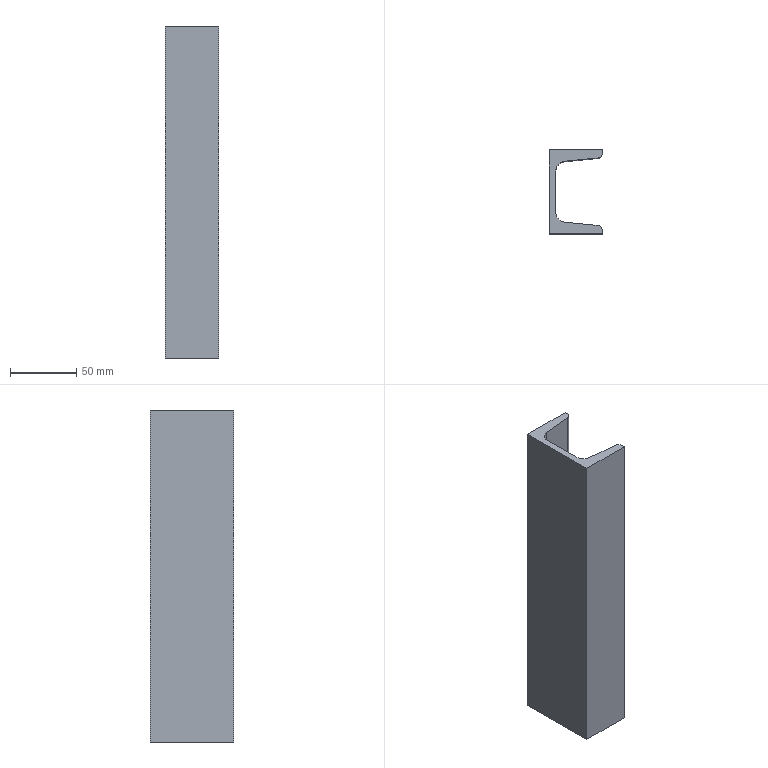Part | STEP file | 750038227 | 1 solid | 14 faces | box 40 x 63 x 250 mm | volume 211142 mm3 | plane 10 | cylinder 4 | commonest cylinder face diameters 7.6 x2 15 x2
STEP:
#1=CARTESIAN_POINT('',(0.,0.,125.));
#2=VERTEX_POINT('',#1);
#3=CARTESIAN_POINT('',(0.,0.,-125.));
#4=VERTEX_POINT('',#3);
#5=CARTESIAN_POINT('',(0.,0.,125.));
#6=DIRECTION('',(0.,0.,-1.));
#7=VECTOR('',#6,1000.);
#8=LINE('',#5,#7);
#9=EDGE_CURVE('',#2,#4,#8,.T.);
#10=ORIENTED_EDGE('',*,*,#9,.F.);
#11=CARTESIAN_POINT('',(0.,63.,125.));
#12=VERTEX_POINT('',#11);
#13=CARTESIAN_POINT('',(0.,63.,125.));
#14=DIRECTION('',(0.,-1.,0.));
#15=VECTOR('',#14,1000.);
#16=LINE('',#13,#15);
#17=EDGE_CURVE('',#12,#2,#16,.T.);
#18=ORIENTED_EDGE('',*,*,#17,.F.);
#19=CARTESIAN_POINT('',(0.,63.,-125.));
#20=VERTEX_POINT('',#19);
#21=CARTESIAN_POINT('',(0.,63.,125.));
#22=DIRECTION('',(0.,0.,1.));
#23=VECTOR('',#22,1000.);
#24=LINE('',#21,#23);
#25=EDGE_CURVE('',#20,#12,#24,.T.);
#26=ORIENTED_EDGE('',*,*,#25,.F.);
#27=CARTESIAN_POINT('',(0.,63.,-125.));
#28=DIRECTION('',(0.,1.,0.));
#29=VECTOR('',#28,1000.);
#30=LINE('',#27,#29);
#31=EDGE_CURVE('',#4,#20,#30,.T.);
#32=ORIENTED_EDGE('',*,*,#31,.F.);
#33=EDGE_LOOP('',(#10,#18,#26,#32));
#34=FACE_OUTER_BOUND('',#33,.T.);
#35=CARTESIAN_POINT('',(0.,63.,125.));
#36=DIRECTION('',(1.,0.,0.));
#37=DIRECTION('',(0.,0.,-1.));
#38=AXIS2_PLACEMENT_3D('',#35,#36,#37);
#39=PLANE('',#38);
#40=ADVANCED_FACE('',(#34),#39,.F.);
#41=CARTESIAN_POINT('',(40.,63.,-125.));
#42=VERTEX_POINT('',#41);
#43=CARTESIAN_POINT('',(36.2,63.,-125.));
#44=DIRECTION('',(-1.,0.,0.));
#45=VECTOR('',#44,1000.);
#46=LINE('',#43,#45);
#47=EDGE_CURVE('',#42,#20,#46,.T.);
#48=ORIENTED_EDGE('',*,*,#47,.F.);
#49=CARTESIAN_POINT('',(40.,60.699,-125.));
#50=VERTEX_POINT('',#49);
#51=CARTESIAN_POINT('',(40.,2.301,-125.));
#52=DIRECTION('',(0.,1.,0.));
#53=VECTOR('',#52,1000.);
#54=LINE('',#51,#53);
#55=EDGE_CURVE('',#50,#42,#54,.T.);
#56=ORIENTED_EDGE('',*,*,#55,.F.);
#57=CARTESIAN_POINT('',(36.578,56.918,-125.));
#58=VERTEX_POINT('',#57);
#59=CARTESIAN_POINT('',(36.2,60.699,-125.));
#60=DIRECTION('',(0.,0.,1.));
#61=DIRECTION('',(-1.,0.,0.));
#62=AXIS2_PLACEMENT_3D('',#59,#60,#61);
#63=CIRCLE('',#62,3.8);
#64=EDGE_CURVE('',#58,#50,#63,.T.);
#65=ORIENTED_EDGE('',*,*,#64,.F.);
#66=CARTESIAN_POINT('',(11.554,54.415,-125.));
#67=VERTEX_POINT('',#66);
#68=CARTESIAN_POINT('',(11.554,54.415,-125.));
#69=DIRECTION('',(0.995,0.0995,0.));
#70=VECTOR('',#69,1000.);
#71=LINE('',#68,#70);
#72=EDGE_CURVE('',#67,#58,#71,.T.);
#73=ORIENTED_EDGE('',*,*,#72,.F.);
#74=CARTESIAN_POINT('',(4.8,46.953,-125.));
#75=VERTEX_POINT('',#74);
#76=CARTESIAN_POINT('',(12.3,46.953,-125.));
#77=DIRECTION('',(0.,0.,-1.));
#78=DIRECTION('',(-1.,0.,0.));
#79=AXIS2_PLACEMENT_3D('',#76,#77,#78);
#80=CIRCLE('',#79,7.5);
#81=EDGE_CURVE('',#75,#67,#80,.T.);
#82=ORIENTED_EDGE('',*,*,#81,.F.);
#83=CARTESIAN_POINT('',(4.8,16.047,-125.));
#84=VERTEX_POINT('',#83);
#85=CARTESIAN_POINT('',(4.8,2.301,-125.));
#86=DIRECTION('',(0.,1.,0.));
#87=VECTOR('',#86,1000.);
#88=LINE('',#85,#87);
#89=EDGE_CURVE('',#84,#75,#88,.T.);
#90=ORIENTED_EDGE('',*,*,#89,.F.);
#91=CARTESIAN_POINT('',(11.554,8.585,-125.));
#92=VERTEX_POINT('',#91);
#93=CARTESIAN_POINT('',(12.3,16.047,-125.));
#94=DIRECTION('',(0.,0.,-1.));
#95=DIRECTION('',(-1.,0.,0.));
#96=AXIS2_PLACEMENT_3D('',#93,#94,#95);
#97=CIRCLE('',#96,7.5);
#98=EDGE_CURVE('',#92,#84,#97,.T.);
#99=ORIENTED_EDGE('',*,*,#98,.F.);
#100=CARTESIAN_POINT('',(36.578,6.082,-125.));
#101=VERTEX_POINT('',#100);
#102=CARTESIAN_POINT('',(36.578,6.082,-125.));
#103=DIRECTION('',(-0.995,0.0995,0.));
#104=VECTOR('',#103,1000.);
#105=LINE('',#102,#104);
#106=EDGE_CURVE('',#101,#92,#105,.T.);
#107=ORIENTED_EDGE('',*,*,#106,.F.);
#108=CARTESIAN_POINT('',(40.,2.301,-125.));
#109=VERTEX_POINT('',#108);
#110=CARTESIAN_POINT('',(36.2,2.301,-125.));
#111=DIRECTION('',(0.,0.,1.));
#112=DIRECTION('',(-1.,0.,0.));
#113=AXIS2_PLACEMENT_3D('',#110,#111,#112);
#114=CIRCLE('',#113,3.8);
#115=EDGE_CURVE('',#109,#101,#114,.T.);
#116=ORIENTED_EDGE('',*,*,#115,.F.);
#117=CARTESIAN_POINT('',(40.,0.,-125.));
#118=VERTEX_POINT('',#117);
#119=CARTESIAN_POINT('',(40.,2.301,-125.));
#120=DIRECTION('',(0.,1.,0.));
#121=VECTOR('',#120,1000.);
#122=LINE('',#119,#121);
#123=EDGE_CURVE('',#118,#109,#122,.T.);
#124=ORIENTED_EDGE('',*,*,#123,.F.);
#125=CARTESIAN_POINT('',(36.2,0.,-125.));
#126=DIRECTION('',(1.,0.,0.));
#127=VECTOR('',#126,1000.);
#128=LINE('',#125,#127);
#129=EDGE_CURVE('',#4,#118,#128,.T.);
#130=ORIENTED_EDGE('',*,*,#129,.F.);
#131=ORIENTED_EDGE('',*,*,#31,.T.);
#132=EDGE_LOOP('',(#48,#56,#65,#73,#82,#90,#99,#107,#116,#124,#130,#131));
#133=FACE_OUTER_BOUND('',#132,.T.);
#134=CARTESIAN_POINT('',(36.2,2.301,-125.));
#135=DIRECTION('',(0.,0.,1.));
#136=DIRECTION('',(1.,0.,0.));
#137=AXIS2_PLACEMENT_3D('',#134,#135,#136);
#138=PLANE('',#137);
#139=ADVANCED_FACE('',(#133),#138,.F.);
#140=CARTESIAN_POINT('',(40.,0.,125.));
#141=VERTEX_POINT('',#140);
#142=CARTESIAN_POINT('',(40.,0.,125.));
#143=DIRECTION('',(0.,0.,-1.));
#144=VECTOR('',#143,1000.);
#145=LINE('',#142,#144);
#146=EDGE_CURVE('',#141,#118,#145,.T.);
#147=ORIENTED_EDGE('',*,*,#146,.F.);
#148=CARTESIAN_POINT('',(0.,0.,125.));
#149=DIRECTION('',(1.,0.,0.));
#150=VECTOR('',#149,1000.);
#151=LINE('',#148,#150);
#152=EDGE_CURVE('',#2,#141,#151,.T.);
#153=ORIENTED_EDGE('',*,*,#152,.F.);
#154=ORIENTED_EDGE('',*,*,#9,.T.);
#155=ORIENTED_EDGE('',*,*,#129,.T.);
#156=EDGE_LOOP('',(#147,#153,#154,#155));
#157=FACE_OUTER_BOUND('',#156,.T.);
#158=CARTESIAN_POINT('',(0.,0.,125.));
#159=DIRECTION('',(0.,1.,0.));
#160=DIRECTION('',(0.,0.,1.));
#161=AXIS2_PLACEMENT_3D('',#158,#159,#160);
#162=PLANE('',#161);
#163=ADVANCED_FACE('',(#157),#162,.F.);
#164=CARTESIAN_POINT('',(40.,60.699,125.));
#165=VERTEX_POINT('',#164);
#166=CARTESIAN_POINT('',(40.,63.,125.));
#167=VERTEX_POINT('',#166);
#168=CARTESIAN_POINT('',(40.,2.301,125.));
#169=DIRECTION('',(0.,1.,0.));
#170=VECTOR('',#169,1000.);
#171=LINE('',#168,#170);
#172=EDGE_CURVE('',#165,#167,#171,.T.);
#173=ORIENTED_EDGE('',*,*,#172,.T.);
#174=CARTESIAN_POINT('',(36.2,63.,125.));
#175=DIRECTION('',(-1.,0.,0.));
#176=VECTOR('',#175,1000.);
#177=LINE('',#174,#176);
#178=EDGE_CURVE('',#167,#12,#177,.T.);
#179=ORIENTED_EDGE('',*,*,#178,.T.);
#180=ORIENTED_EDGE('',*,*,#17,.T.);
#181=ORIENTED_EDGE('',*,*,#152,.T.);
#182=CARTESIAN_POINT('',(40.,2.301,125.));
#183=VERTEX_POINT('',#182);
#184=CARTESIAN_POINT('',(40.,2.301,125.));
#185=DIRECTION('',(0.,1.,0.));
#186=VECTOR('',#185,1000.);
#187=LINE('',#184,#186);
#188=EDGE_CURVE('',#141,#183,#187,.T.);
#189=ORIENTED_EDGE('',*,*,#188,.T.);
#190=CARTESIAN_POINT('',(36.578,6.082,125.));
#191=VERTEX_POINT('',#190);
#192=CARTESIAN_POINT('',(36.2,2.301,125.));
#193=DIRECTION('',(0.,0.,1.));
#194=DIRECTION('',(-1.,0.,0.));
#195=AXIS2_PLACEMENT_3D('',#192,#193,#194);
#196=CIRCLE('',#195,3.8);
#197=EDGE_CURVE('',#183,#191,#196,.T.);
#198=ORIENTED_EDGE('',*,*,#197,.T.);
#199=CARTESIAN_POINT('',(11.554,8.585,125.));
#200=VERTEX_POINT('',#199);
#201=CARTESIAN_POINT('',(36.578,6.082,125.));
#202=DIRECTION('',(-0.995,0.0995,0.));
#203=VECTOR('',#202,1000.);
#204=LINE('',#201,#203);
#205=EDGE_CURVE('',#191,#200,#204,.T.);
#206=ORIENTED_EDGE('',*,*,#205,.T.);
#207=CARTESIAN_POINT('',(4.8,16.047,125.));
#208=VERTEX_POINT('',#207);
#209=CARTESIAN_POINT('',(12.3,16.047,125.));
#210=DIRECTION('',(0.,0.,-1.));
#211=DIRECTION('',(-1.,0.,0.));
#212=AXIS2_PLACEMENT_3D('',#209,#210,#211);
#213=CIRCLE('',#212,7.5);
#214=EDGE_CURVE('',#200,#208,#213,.T.);
#215=ORIENTED_EDGE('',*,*,#214,.T.);
#216=CARTESIAN_POINT('',(4.8,46.953,125.));
#217=VERTEX_POINT('',#216);
#218=CARTESIAN_POINT('',(4.8,2.301,125.));
#219=DIRECTION('',(0.,1.,0.));
#220=VECTOR('',#219,1000.);
#221=LINE('',#218,#220);
#222=EDGE_CURVE('',#208,#217,#221,.T.);
#223=ORIENTED_EDGE('',*,*,#222,.T.);
#224=CARTESIAN_POINT('',(11.554,54.415,125.));
#225=VERTEX_POINT('',#224);
#226=CARTESIAN_POINT('',(12.3,46.953,125.));
#227=DIRECTION('',(0.,0.,-1.));
#228=DIRECTION('',(-1.,0.,0.));
#229=AXIS2_PLACEMENT_3D('',#226,#227,#228);
#230=CIRCLE('',#229,7.5);
#231=EDGE_CURVE('',#217,#225,#230,.T.);
#232=ORIENTED_EDGE('',*,*,#231,.T.);
#233=CARTESIAN_POINT('',(36.578,56.918,125.));
#234=VERTEX_POINT('',#233);
#235=CARTESIAN_POINT('',(11.554,54.415,125.));
#236=DIRECTION('',(0.995,0.0995,0.));
#237=VECTOR('',#236,1000.);
#238=LINE('',#235,#237);
#239=EDGE_CURVE('',#225,#234,#238,.T.);
#240=ORIENTED_EDGE('',*,*,#239,.T.);
#241=CARTESIAN_POINT('',(36.2,60.699,125.));
#242=DIRECTION('',(0.,0.,1.));
#243=DIRECTION('',(-1.,0.,0.));
#244=AXIS2_PLACEMENT_3D('',#241,#242,#243);
#245=CIRCLE('',#244,3.8);
#246=EDGE_CURVE('',#234,#165,#245,.T.);
#247=ORIENTED_EDGE('',*,*,#246,.T.);
#248=EDGE_LOOP('',(#173,#179,#180,#181,#189,#198,#206,#215,#223,#232,#240,#247));
#249=FACE_OUTER_BOUND('',#248,.T.);
#250=CARTESIAN_POINT('',(36.2,2.301,125.));
#251=DIRECTION('',(0.,0.,1.));
#252=DIRECTION('',(1.,0.,0.));
#253=AXIS2_PLACEMENT_3D('',#250,#251,#252);
#254=PLANE('',#253);
#255=ADVANCED_FACE('',(#249),#254,.T.);
#256=ORIENTED_EDGE('',*,*,#25,.T.);
#257=ORIENTED_EDGE('',*,*,#178,.F.);
#258=CARTESIAN_POINT('',(40.,63.,125.));
#259=DIRECTION('',(0.,0.,1.));
#260=VECTOR('',#259,1000.);
#261=LINE('',#258,#260);
#262=EDGE_CURVE('',#42,#167,#261,.T.);
#263=ORIENTED_EDGE('',*,*,#262,.F.);
#264=ORIENTED_EDGE('',*,*,#47,.T.);
#265=EDGE_LOOP('',(#256,#257,#263,#264));
#266=FACE_OUTER_BOUND('',#265,.T.);
#267=CARTESIAN_POINT('',(40.,63.,125.));
#268=DIRECTION('',(0.,-1.,0.));
#269=DIRECTION('',(0.,0.,-1.));
#270=AXIS2_PLACEMENT_3D('',#267,#268,#269);
#271=PLANE('',#270);
#272=ADVANCED_FACE('',(#266),#271,.F.);
#273=ORIENTED_EDGE('',*,*,#262,.T.);
#274=ORIENTED_EDGE('',*,*,#172,.F.);
#275=CARTESIAN_POINT('',(40.,60.699,125.));
#276=DIRECTION('',(0.,0.,1.));
#277=VECTOR('',#276,1000.);
#278=LINE('',#275,#277);
#279=EDGE_CURVE('',#50,#165,#278,.T.);
#280=ORIENTED_EDGE('',*,*,#279,.F.);
#281=ORIENTED_EDGE('',*,*,#55,.T.);
#282=EDGE_LOOP('',(#273,#274,#280,#281));
#283=FACE_OUTER_BOUND('',#282,.T.);
#284=CARTESIAN_POINT('',(40.,60.699,125.));
#285=DIRECTION('',(-1.,0.,0.));
#286=DIRECTION('',(0.,-1.,0.));
#287=AXIS2_PLACEMENT_3D('',#284,#285,#286);
#288=PLANE('',#287);
#289=ADVANCED_FACE('',(#283),#288,.F.);
#290=ORIENTED_EDGE('',*,*,#246,.F.);
#291=CARTESIAN_POINT('',(36.578,56.918,125.));
#292=DIRECTION('',(0.,0.,-1.));
#293=VECTOR('',#292,1000.);
#294=LINE('',#291,#293);
#295=EDGE_CURVE('',#234,#58,#294,.T.);
#296=ORIENTED_EDGE('',*,*,#295,.T.);
#297=ORIENTED_EDGE('',*,*,#64,.T.);
#298=ORIENTED_EDGE('',*,*,#279,.T.);
#299=EDGE_LOOP('',(#290,#296,#297,#298));
#300=FACE_OUTER_BOUND('',#299,.T.);
#301=CARTESIAN_POINT('',(36.2,60.699,125.));
#302=DIRECTION('',(0.,0.,-1.));
#303=DIRECTION('',(-1.,0.,0.));
#304=AXIS2_PLACEMENT_3D('',#301,#302,#303);
#305=CYLINDRICAL_SURFACE('',#304,3.8);
#306=ADVANCED_FACE('',(#300),#305,.T.);
#307=ORIENTED_EDGE('',*,*,#295,.F.);
#308=ORIENTED_EDGE('',*,*,#239,.F.);
#309=CARTESIAN_POINT('',(11.554,54.415,125.));
#310=DIRECTION('',(0.,0.,1.));
#311=VECTOR('',#310,1000.);
#312=LINE('',#309,#311);
#313=EDGE_CURVE('',#67,#225,#312,.T.);
#314=ORIENTED_EDGE('',*,*,#313,.F.);
#315=ORIENTED_EDGE('',*,*,#72,.T.);
#316=EDGE_LOOP('',(#307,#308,#314,#315));
#317=FACE_OUTER_BOUND('',#316,.T.);
#318=CARTESIAN_POINT('',(11.554,54.415,125.));
#319=DIRECTION('',(-0.0995,0.995,0.));
#320=DIRECTION('',(-0.995,-0.0995,0.));
#321=AXIS2_PLACEMENT_3D('',#318,#319,#320);
#322=PLANE('',#321);
#323=ADVANCED_FACE('',(#317),#322,.F.);
#324=ORIENTED_EDGE('',*,*,#313,.T.);
#325=ORIENTED_EDGE('',*,*,#231,.F.);
#326=CARTESIAN_POINT('',(4.8,46.953,125.));
#327=DIRECTION('',(0.,0.,1.));
#328=VECTOR('',#327,1000.);
#329=LINE('',#326,#328);
#330=EDGE_CURVE('',#75,#217,#329,.T.);
#331=ORIENTED_EDGE('',*,*,#330,.F.);
#332=ORIENTED_EDGE('',*,*,#81,.T.);
#333=EDGE_LOOP('',(#324,#325,#331,#332));
#334=FACE_OUTER_BOUND('',#333,.T.);
#335=CARTESIAN_POINT('',(12.3,46.953,125.));
#336=DIRECTION('',(0.,0.,-1.));
#337=DIRECTION('',(-1.,0.,0.));
#338=AXIS2_PLACEMENT_3D('',#335,#336,#337);
#339=CYLINDRICAL_SURFACE('',#338,7.5);
#340=ADVANCED_FACE('',(#334),#339,.F.);
#341=ORIENTED_EDGE('',*,*,#330,.T.);
#342=ORIENTED_EDGE('',*,*,#222,.F.);
#343=CARTESIAN_POINT('',(4.8,16.047,125.));
#344=DIRECTION('',(0.,0.,1.));
#345=VECTOR('',#344,1000.);
#346=LINE('',#343,#345);
#347=EDGE_CURVE('',#84,#208,#346,.T.);
#348=ORIENTED_EDGE('',*,*,#347,.F.);
#349=ORIENTED_EDGE('',*,*,#89,.T.);
#350=EDGE_LOOP('',(#341,#342,#348,#349));
#351=FACE_OUTER_BOUND('',#350,.T.);
#352=CARTESIAN_POINT('',(4.8,16.047,125.));
#353=DIRECTION('',(-1.,0.,0.));
#354=DIRECTION('',(0.,-1.,0.));
#355=AXIS2_PLACEMENT_3D('',#352,#353,#354);
#356=PLANE('',#355);
#357=ADVANCED_FACE('',(#351),#356,.F.);
#358=ORIENTED_EDGE('',*,*,#347,.T.);
#359=ORIENTED_EDGE('',*,*,#214,.F.);
#360=CARTESIAN_POINT('',(11.554,8.585,125.));
#361=DIRECTION('',(0.,0.,1.));
#362=VECTOR('',#361,1000.);
#363=LINE('',#360,#362);
#364=EDGE_CURVE('',#92,#200,#363,.T.);
#365=ORIENTED_EDGE('',*,*,#364,.F.);
#366=ORIENTED_EDGE('',*,*,#98,.T.);
#367=EDGE_LOOP('',(#358,#359,#365,#366));
#368=FACE_OUTER_BOUND('',#367,.T.);
#369=CARTESIAN_POINT('',(12.3,16.047,125.));
#370=DIRECTION('',(0.,0.,-1.));
#371=DIRECTION('',(-1.,0.,0.));
#372=AXIS2_PLACEMENT_3D('',#369,#370,#371);
#373=CYLINDRICAL_SURFACE('',#372,7.5);
#374=ADVANCED_FACE('',(#368),#373,.F.);
#375=ORIENTED_EDGE('',*,*,#364,.T.);
#376=ORIENTED_EDGE('',*,*,#205,.F.);
#377=CARTESIAN_POINT('',(36.578,6.082,125.));
#378=DIRECTION('',(0.,0.,1.));
#379=VECTOR('',#378,1000.);
#380=LINE('',#377,#379);
#381=EDGE_CURVE('',#101,#191,#380,.T.);
#382=ORIENTED_EDGE('',*,*,#381,.F.);
#383=ORIENTED_EDGE('',*,*,#106,.T.);
#384=EDGE_LOOP('',(#375,#376,#382,#383));
#385=FACE_OUTER_BOUND('',#384,.T.);
#386=CARTESIAN_POINT('',(36.578,6.082,125.));
#387=DIRECTION('',(-0.0995,-0.995,0.));
#388=DIRECTION('',(0.995,-0.0995,0.));
#389=AXIS2_PLACEMENT_3D('',#386,#387,#388);
#390=PLANE('',#389);
#391=ADVANCED_FACE('',(#385),#390,.F.);
#392=ORIENTED_EDGE('',*,*,#197,.F.);
#393=CARTESIAN_POINT('',(40.,2.301,125.));
#394=DIRECTION('',(0.,0.,-1.));
#395=VECTOR('',#394,1000.);
#396=LINE('',#393,#395);
#397=EDGE_CURVE('',#183,#109,#396,.T.);
#398=ORIENTED_EDGE('',*,*,#397,.T.);
#399=ORIENTED_EDGE('',*,*,#115,.T.);
#400=ORIENTED_EDGE('',*,*,#381,.T.);
#401=EDGE_LOOP('',(#392,#398,#399,#400));
#402=FACE_OUTER_BOUND('',#401,.T.);
#403=CARTESIAN_POINT('',(36.2,2.301,125.));
#404=DIRECTION('',(0.,0.,-1.));
#405=DIRECTION('',(-1.,0.,0.));
#406=AXIS2_PLACEMENT_3D('',#403,#404,#405);
#407=CYLINDRICAL_SURFACE('',#406,3.8);
#408=ADVANCED_FACE('',(#402),#407,.T.);
#409=ORIENTED_EDGE('',*,*,#397,.F.);
#410=ORIENTED_EDGE('',*,*,#188,.F.);
#411=ORIENTED_EDGE('',*,*,#146,.T.);
#412=ORIENTED_EDGE('',*,*,#123,.T.);
#413=EDGE_LOOP('',(#409,#410,#411,#412));
#414=FACE_OUTER_BOUND('',#413,.T.);
#415=CARTESIAN_POINT('',(40.,0.,125.));
#416=DIRECTION('',(-1.,0.,0.));
#417=DIRECTION('',(0.,0.,1.));
#418=AXIS2_PLACEMENT_3D('',#415,#416,#417);
#419=PLANE('',#418);
#420=ADVANCED_FACE('',(#414),#419,.F.);
#421=CLOSED_SHELL('',(#40,#139,#163,#255,#272,#289,#306,#323,#340,#357,#374,#391,#408,#420));
#422=MANIFOLD_SOLID_BREP('',#421);
#423=CARTESIAN_POINT('',(0.,0.,0.));
#424=DIRECTION('',(0.,0.,1.));
#425=DIRECTION('',(1.,0.,0.));
#426=AXIS2_PLACEMENT_3D('',#423,#424,#425);
#427=(LENGTH_UNIT()NAMED_UNIT(*)SI_UNIT(.MILLI.,.METRE.));
#428=UNCERTAINTY_MEASURE_WITH_UNIT(LENGTH_MEASURE(0.00001),#427,'','');
#429=(NAMED_UNIT(*)PLANE_ANGLE_UNIT()SI_UNIT($,.RADIAN.));
#430=(NAMED_UNIT(*)SI_UNIT($,.STERADIAN.)SOLID_ANGLE_UNIT());
#431=(GEOMETRIC_REPRESENTATION_CONTEXT(3)GLOBAL_UNCERTAINTY_ASSIGNED_CONTEXT((#428))GLOBAL_UNIT_ASSIGNED_CONTEXT((#427,#429,#430))REPRESENTATION_CONTEXT('',''));
#432=ADVANCED_BREP_SHAPE_REPRESENTATION('',(#422,#426),#431);